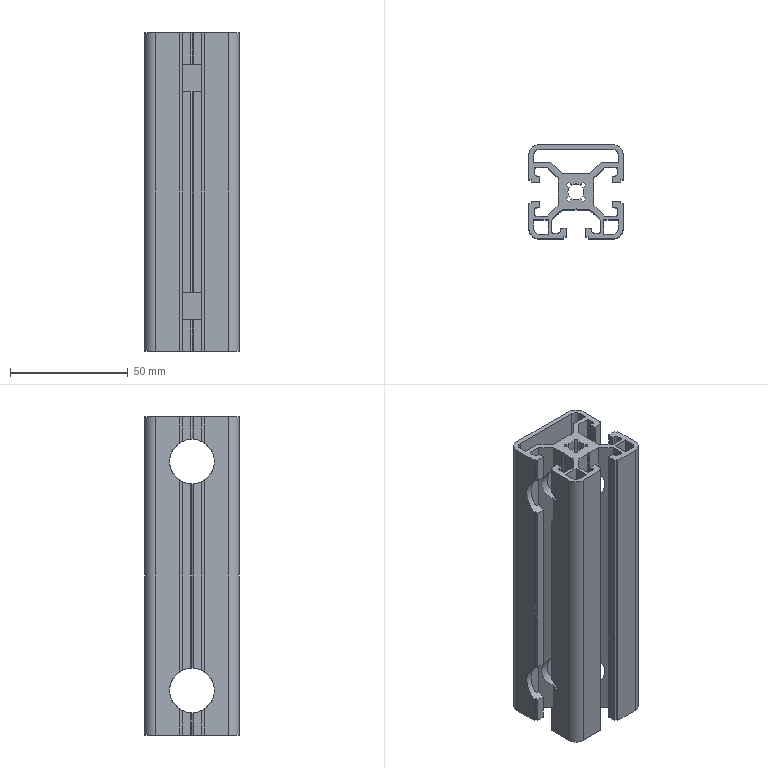Part | SolidWorks | features BaseBody 1, HoleWzd 1, MoveFace 1 | 1 solid | 242 faces | box 40 x 40 x 135 mm | volume 71545 mm3 | plane 187 | cylinder 55 | commonest cylinder face diameters 6.8 x15 2 x14 19 x12 1 x6 5 x4 9 x4